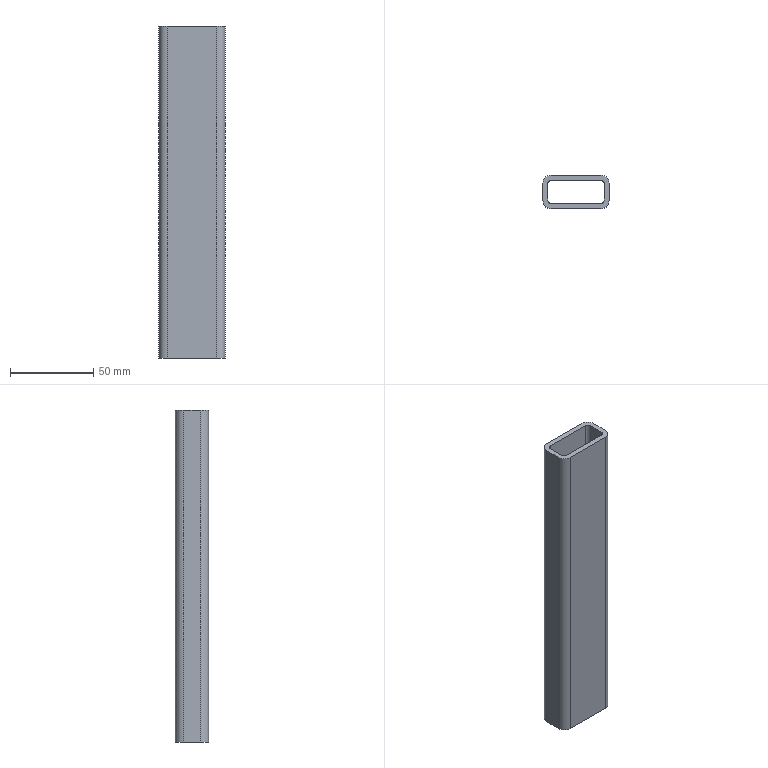Part | SolidWorks | features Extrusion 1 | 1 solid | 18 faces | box 40 x 20 x 200 mm | volume 61195 mm3 | plane 10 | cylinder 8 | commonest cylinder face diameters 4 x4 10 x4
STEP:
#1=CARTESIAN_POINT('',(35.,0.,200.));
#2=VERTEX_POINT('',#1);
#3=CARTESIAN_POINT('',(40.,5.,200.));
#4=VERTEX_POINT('',#3);
#5=CARTESIAN_POINT('',(35.,5.,200.));
#6=DIRECTION('',(0.,0.,1.));
#7=DIRECTION('',(1.,0.,0.));
#8=AXIS2_PLACEMENT_3D('',#5,#6,#7);
#9=CIRCLE('',#8,5.);
#10=EDGE_CURVE('',#2,#4,#9,.T.);
#11=ORIENTED_EDGE('',*,*,#10,.T.);
#12=CARTESIAN_POINT('',(40.,15.,200.));
#13=VERTEX_POINT('',#12);
#14=CARTESIAN_POINT('',(40.,5.,200.));
#15=DIRECTION('',(0.,1.,0.));
#16=VECTOR('',#15,1000.);
#17=LINE('',#14,#16);
#18=EDGE_CURVE('',#4,#13,#17,.T.);
#19=ORIENTED_EDGE('',*,*,#18,.T.);
#20=CARTESIAN_POINT('',(35.,20.,200.));
#21=VERTEX_POINT('',#20);
#22=CARTESIAN_POINT('',(35.,15.,200.));
#23=DIRECTION('',(0.,0.,1.));
#24=DIRECTION('',(-1.,0.,0.));
#25=AXIS2_PLACEMENT_3D('',#22,#23,#24);
#26=CIRCLE('',#25,5.);
#27=EDGE_CURVE('',#13,#21,#26,.T.);
#28=ORIENTED_EDGE('',*,*,#27,.T.);
#29=CARTESIAN_POINT('',(5.,20.,200.));
#30=VERTEX_POINT('',#29);
#31=CARTESIAN_POINT('',(5.,20.,200.));
#32=DIRECTION('',(-1.,0.,0.));
#33=VECTOR('',#32,1000.);
#34=LINE('',#31,#33);
#35=EDGE_CURVE('',#21,#30,#34,.T.);
#36=ORIENTED_EDGE('',*,*,#35,.T.);
#37=CARTESIAN_POINT('',(0.,15.,200.));
#38=VERTEX_POINT('',#37);
#39=CARTESIAN_POINT('',(5.,15.,200.));
#40=DIRECTION('',(0.,0.,1.));
#41=DIRECTION('',(-1.,0.,0.));
#42=AXIS2_PLACEMENT_3D('',#39,#40,#41);
#43=CIRCLE('',#42,5.);
#44=EDGE_CURVE('',#30,#38,#43,.T.);
#45=ORIENTED_EDGE('',*,*,#44,.T.);
#46=CARTESIAN_POINT('',(0.,5.,200.));
#47=VERTEX_POINT('',#46);
#48=CARTESIAN_POINT('',(0.,5.,200.));
#49=DIRECTION('',(0.,-1.,0.));
#50=VECTOR('',#49,1000.);
#51=LINE('',#48,#50);
#52=EDGE_CURVE('',#38,#47,#51,.T.);
#53=ORIENTED_EDGE('',*,*,#52,.T.);
#54=CARTESIAN_POINT('',(5.,0.,200.));
#55=VERTEX_POINT('',#54);
#56=CARTESIAN_POINT('',(5.,5.,200.));
#57=DIRECTION('',(0.,0.,1.));
#58=DIRECTION('',(-1.,0.,0.));
#59=AXIS2_PLACEMENT_3D('',#56,#57,#58);
#60=CIRCLE('',#59,5.);
#61=EDGE_CURVE('',#47,#55,#60,.T.);
#62=ORIENTED_EDGE('',*,*,#61,.T.);
#63=CARTESIAN_POINT('',(5.,0.,200.));
#64=DIRECTION('',(1.,0.,0.));
#65=VECTOR('',#64,1000.);
#66=LINE('',#63,#65);
#67=EDGE_CURVE('',#55,#2,#66,.T.);
#68=ORIENTED_EDGE('',*,*,#67,.T.);
#69=EDGE_LOOP('',(#11,#19,#28,#36,#45,#53,#62,#68));
#70=FACE_OUTER_BOUND('',#69,.T.);
#71=CARTESIAN_POINT('',(3.,15.,200.));
#72=VERTEX_POINT('',#71);
#73=CARTESIAN_POINT('',(3.,5.,200.));
#74=VERTEX_POINT('',#73);
#75=CARTESIAN_POINT('',(3.,5.,200.));
#76=DIRECTION('',(0.,-1.,0.));
#77=VECTOR('',#76,1000.);
#78=LINE('',#75,#77);
#79=EDGE_CURVE('',#72,#74,#78,.T.);
#80=ORIENTED_EDGE('',*,*,#79,.F.);
#81=CARTESIAN_POINT('',(5.,17.,200.));
#82=VERTEX_POINT('',#81);
#83=CARTESIAN_POINT('',(5.,15.,200.));
#84=DIRECTION('',(0.,0.,1.));
#85=DIRECTION('',(-1.,0.,0.));
#86=AXIS2_PLACEMENT_3D('',#83,#84,#85);
#87=CIRCLE('',#86,2.);
#88=EDGE_CURVE('',#82,#72,#87,.T.);
#89=ORIENTED_EDGE('',*,*,#88,.F.);
#90=CARTESIAN_POINT('',(35.,17.,200.));
#91=VERTEX_POINT('',#90);
#92=CARTESIAN_POINT('',(5.,17.,200.));
#93=DIRECTION('',(-1.,0.,0.));
#94=VECTOR('',#93,1000.);
#95=LINE('',#92,#94);
#96=EDGE_CURVE('',#91,#82,#95,.T.);
#97=ORIENTED_EDGE('',*,*,#96,.F.);
#98=CARTESIAN_POINT('',(37.,15.,200.));
#99=VERTEX_POINT('',#98);
#100=CARTESIAN_POINT('',(35.,15.,200.));
#101=DIRECTION('',(0.,0.,1.));
#102=DIRECTION('',(-1.,0.,0.));
#103=AXIS2_PLACEMENT_3D('',#100,#101,#102);
#104=CIRCLE('',#103,2.);
#105=EDGE_CURVE('',#99,#91,#104,.T.);
#106=ORIENTED_EDGE('',*,*,#105,.F.);
#107=CARTESIAN_POINT('',(37.,5.,200.));
#108=VERTEX_POINT('',#107);
#109=CARTESIAN_POINT('',(37.,5.,200.));
#110=DIRECTION('',(0.,1.,0.));
#111=VECTOR('',#110,1000.);
#112=LINE('',#109,#111);
#113=EDGE_CURVE('',#108,#99,#112,.T.);
#114=ORIENTED_EDGE('',*,*,#113,.F.);
#115=CARTESIAN_POINT('',(35.,3.,200.));
#116=VERTEX_POINT('',#115);
#117=CARTESIAN_POINT('',(35.,5.,200.));
#118=DIRECTION('',(0.,0.,1.));
#119=DIRECTION('',(1.,0.,0.));
#120=AXIS2_PLACEMENT_3D('',#117,#118,#119);
#121=CIRCLE('',#120,2.);
#122=EDGE_CURVE('',#116,#108,#121,.T.);
#123=ORIENTED_EDGE('',*,*,#122,.F.);
#124=CARTESIAN_POINT('',(5.,3.,200.));
#125=VERTEX_POINT('',#124);
#126=CARTESIAN_POINT('',(5.,3.,200.));
#127=DIRECTION('',(1.,0.,0.));
#128=VECTOR('',#127,1000.);
#129=LINE('',#126,#128);
#130=EDGE_CURVE('',#125,#116,#129,.T.);
#131=ORIENTED_EDGE('',*,*,#130,.F.);
#132=CARTESIAN_POINT('',(5.,5.,200.));
#133=DIRECTION('',(0.,0.,1.));
#134=DIRECTION('',(-1.,0.,0.));
#135=AXIS2_PLACEMENT_3D('',#132,#133,#134);
#136=CIRCLE('',#135,2.);
#137=EDGE_CURVE('',#74,#125,#136,.T.);
#138=ORIENTED_EDGE('',*,*,#137,.F.);
#139=EDGE_LOOP('',(#80,#89,#97,#106,#114,#123,#131,#138));
#140=FACE_BOUND('',#139,.T.);
#141=CARTESIAN_POINT('',(35.,5.,200.));
#142=DIRECTION('',(0.,0.,1.));
#143=DIRECTION('',(1.,0.,0.));
#144=AXIS2_PLACEMENT_3D('',#141,#142,#143);
#145=PLANE('',#144);
#146=ADVANCED_FACE('',(#70,#140),#145,.T.);
#147=CARTESIAN_POINT('',(35.,0.,0.));
#148=VERTEX_POINT('',#147);
#149=CARTESIAN_POINT('',(40.,5.,0.));
#150=VERTEX_POINT('',#149);
#151=CARTESIAN_POINT('',(35.,5.,0.));
#152=DIRECTION('',(0.,0.,1.));
#153=DIRECTION('',(1.,0.,0.));
#154=AXIS2_PLACEMENT_3D('',#151,#152,#153);
#155=CIRCLE('',#154,5.);
#156=EDGE_CURVE('',#148,#150,#155,.T.);
#157=ORIENTED_EDGE('',*,*,#156,.F.);
#158=CARTESIAN_POINT('',(5.,0.,0.));
#159=VERTEX_POINT('',#158);
#160=CARTESIAN_POINT('',(5.,0.,0.));
#161=DIRECTION('',(1.,0.,0.));
#162=VECTOR('',#161,1000.);
#163=LINE('',#160,#162);
#164=EDGE_CURVE('',#159,#148,#163,.T.);
#165=ORIENTED_EDGE('',*,*,#164,.F.);
#166=CARTESIAN_POINT('',(0.,5.,0.));
#167=VERTEX_POINT('',#166);
#168=CARTESIAN_POINT('',(5.,5.,0.));
#169=DIRECTION('',(0.,0.,1.));
#170=DIRECTION('',(-1.,0.,0.));
#171=AXIS2_PLACEMENT_3D('',#168,#169,#170);
#172=CIRCLE('',#171,5.);
#173=EDGE_CURVE('',#167,#159,#172,.T.);
#174=ORIENTED_EDGE('',*,*,#173,.F.);
#175=CARTESIAN_POINT('',(0.,15.,0.));
#176=VERTEX_POINT('',#175);
#177=CARTESIAN_POINT('',(0.,5.,0.));
#178=DIRECTION('',(0.,-1.,0.));
#179=VECTOR('',#178,1000.);
#180=LINE('',#177,#179);
#181=EDGE_CURVE('',#176,#167,#180,.T.);
#182=ORIENTED_EDGE('',*,*,#181,.F.);
#183=CARTESIAN_POINT('',(5.,20.,0.));
#184=VERTEX_POINT('',#183);
#185=CARTESIAN_POINT('',(5.,15.,0.));
#186=DIRECTION('',(0.,0.,1.));
#187=DIRECTION('',(-1.,0.,0.));
#188=AXIS2_PLACEMENT_3D('',#185,#186,#187);
#189=CIRCLE('',#188,5.);
#190=EDGE_CURVE('',#184,#176,#189,.T.);
#191=ORIENTED_EDGE('',*,*,#190,.F.);
#192=CARTESIAN_POINT('',(35.,20.,0.));
#193=VERTEX_POINT('',#192);
#194=CARTESIAN_POINT('',(5.,20.,0.));
#195=DIRECTION('',(-1.,0.,0.));
#196=VECTOR('',#195,1000.);
#197=LINE('',#194,#196);
#198=EDGE_CURVE('',#193,#184,#197,.T.);
#199=ORIENTED_EDGE('',*,*,#198,.F.);
#200=CARTESIAN_POINT('',(40.,15.,0.));
#201=VERTEX_POINT('',#200);
#202=CARTESIAN_POINT('',(35.,15.,0.));
#203=DIRECTION('',(0.,0.,1.));
#204=DIRECTION('',(-1.,0.,0.));
#205=AXIS2_PLACEMENT_3D('',#202,#203,#204);
#206=CIRCLE('',#205,5.);
#207=EDGE_CURVE('',#201,#193,#206,.T.);
#208=ORIENTED_EDGE('',*,*,#207,.F.);
#209=CARTESIAN_POINT('',(40.,5.,0.));
#210=DIRECTION('',(0.,1.,0.));
#211=VECTOR('',#210,1000.);
#212=LINE('',#209,#211);
#213=EDGE_CURVE('',#150,#201,#212,.T.);
#214=ORIENTED_EDGE('',*,*,#213,.F.);
#215=EDGE_LOOP('',(#157,#165,#174,#182,#191,#199,#208,#214));
#216=FACE_OUTER_BOUND('',#215,.T.);
#217=CARTESIAN_POINT('',(5.,17.,0.));
#218=VERTEX_POINT('',#217);
#219=CARTESIAN_POINT('',(3.,15.,0.));
#220=VERTEX_POINT('',#219);
#221=CARTESIAN_POINT('',(5.,15.,0.));
#222=DIRECTION('',(0.,0.,1.));
#223=DIRECTION('',(-1.,0.,0.));
#224=AXIS2_PLACEMENT_3D('',#221,#222,#223);
#225=CIRCLE('',#224,2.);
#226=EDGE_CURVE('',#218,#220,#225,.T.);
#227=ORIENTED_EDGE('',*,*,#226,.T.);
#228=CARTESIAN_POINT('',(3.,5.,0.));
#229=VERTEX_POINT('',#228);
#230=CARTESIAN_POINT('',(3.,5.,0.));
#231=DIRECTION('',(0.,-1.,0.));
#232=VECTOR('',#231,1000.);
#233=LINE('',#230,#232);
#234=EDGE_CURVE('',#220,#229,#233,.T.);
#235=ORIENTED_EDGE('',*,*,#234,.T.);
#236=CARTESIAN_POINT('',(5.,3.,0.));
#237=VERTEX_POINT('',#236);
#238=CARTESIAN_POINT('',(5.,5.,0.));
#239=DIRECTION('',(0.,0.,1.));
#240=DIRECTION('',(-1.,0.,0.));
#241=AXIS2_PLACEMENT_3D('',#238,#239,#240);
#242=CIRCLE('',#241,2.);
#243=EDGE_CURVE('',#229,#237,#242,.T.);
#244=ORIENTED_EDGE('',*,*,#243,.T.);
#245=CARTESIAN_POINT('',(35.,3.,0.));
#246=VERTEX_POINT('',#245);
#247=CARTESIAN_POINT('',(5.,3.,0.));
#248=DIRECTION('',(1.,0.,0.));
#249=VECTOR('',#248,1000.);
#250=LINE('',#247,#249);
#251=EDGE_CURVE('',#237,#246,#250,.T.);
#252=ORIENTED_EDGE('',*,*,#251,.T.);
#253=CARTESIAN_POINT('',(37.,5.,0.));
#254=VERTEX_POINT('',#253);
#255=CARTESIAN_POINT('',(35.,5.,0.));
#256=DIRECTION('',(0.,0.,1.));
#257=DIRECTION('',(1.,0.,0.));
#258=AXIS2_PLACEMENT_3D('',#255,#256,#257);
#259=CIRCLE('',#258,2.);
#260=EDGE_CURVE('',#246,#254,#259,.T.);
#261=ORIENTED_EDGE('',*,*,#260,.T.);
#262=CARTESIAN_POINT('',(37.,15.,0.));
#263=VERTEX_POINT('',#262);
#264=CARTESIAN_POINT('',(37.,5.,0.));
#265=DIRECTION('',(0.,1.,0.));
#266=VECTOR('',#265,1000.);
#267=LINE('',#264,#266);
#268=EDGE_CURVE('',#254,#263,#267,.T.);
#269=ORIENTED_EDGE('',*,*,#268,.T.);
#270=CARTESIAN_POINT('',(35.,17.,0.));
#271=VERTEX_POINT('',#270);
#272=CARTESIAN_POINT('',(35.,15.,0.));
#273=DIRECTION('',(0.,0.,1.));
#274=DIRECTION('',(-1.,0.,0.));
#275=AXIS2_PLACEMENT_3D('',#272,#273,#274);
#276=CIRCLE('',#275,2.);
#277=EDGE_CURVE('',#263,#271,#276,.T.);
#278=ORIENTED_EDGE('',*,*,#277,.T.);
#279=CARTESIAN_POINT('',(5.,17.,0.));
#280=DIRECTION('',(-1.,0.,0.));
#281=VECTOR('',#280,1000.);
#282=LINE('',#279,#281);
#283=EDGE_CURVE('',#271,#218,#282,.T.);
#284=ORIENTED_EDGE('',*,*,#283,.T.);
#285=EDGE_LOOP('',(#227,#235,#244,#252,#261,#269,#278,#284));
#286=FACE_BOUND('',#285,.T.);
#287=CARTESIAN_POINT('',(35.,5.,0.));
#288=DIRECTION('',(0.,0.,1.));
#289=DIRECTION('',(1.,0.,0.));
#290=AXIS2_PLACEMENT_3D('',#287,#288,#289);
#291=PLANE('',#290);
#292=ADVANCED_FACE('',(#216,#286),#291,.F.);
#293=ORIENTED_EDGE('',*,*,#156,.T.);
#294=CARTESIAN_POINT('',(40.,5.,200.));
#295=DIRECTION('',(0.,0.,-1.));
#296=VECTOR('',#295,1000.);
#297=LINE('',#294,#296);
#298=EDGE_CURVE('',#4,#150,#297,.T.);
#299=ORIENTED_EDGE('',*,*,#298,.F.);
#300=ORIENTED_EDGE('',*,*,#10,.F.);
#301=CARTESIAN_POINT('',(35.,0.,200.));
#302=DIRECTION('',(0.,0.,-1.));
#303=VECTOR('',#302,1000.);
#304=LINE('',#301,#303);
#305=EDGE_CURVE('',#2,#148,#304,.T.);
#306=ORIENTED_EDGE('',*,*,#305,.T.);
#307=EDGE_LOOP('',(#293,#299,#300,#306));
#308=FACE_OUTER_BOUND('',#307,.T.);
#309=CARTESIAN_POINT('',(35.,5.,200.));
#310=DIRECTION('',(0.,0.,-1.));
#311=DIRECTION('',(-1.,0.,0.));
#312=AXIS2_PLACEMENT_3D('',#309,#310,#311);
#313=CYLINDRICAL_SURFACE('',#312,5.);
#314=ADVANCED_FACE('',(#308),#313,.T.);
#315=ORIENTED_EDGE('',*,*,#213,.T.);
#316=CARTESIAN_POINT('',(40.,15.,200.));
#317=DIRECTION('',(0.,0.,-1.));
#318=VECTOR('',#317,1000.);
#319=LINE('',#316,#318);
#320=EDGE_CURVE('',#13,#201,#319,.T.);
#321=ORIENTED_EDGE('',*,*,#320,.F.);
#322=ORIENTED_EDGE('',*,*,#18,.F.);
#323=ORIENTED_EDGE('',*,*,#298,.T.);
#324=EDGE_LOOP('',(#315,#321,#322,#323));
#325=FACE_OUTER_BOUND('',#324,.T.);
#326=CARTESIAN_POINT('',(40.,5.,200.));
#327=DIRECTION('',(-1.,0.,0.));
#328=DIRECTION('',(0.,0.,1.));
#329=AXIS2_PLACEMENT_3D('',#326,#327,#328);
#330=PLANE('',#329);
#331=ADVANCED_FACE('',(#325),#330,.F.);
#332=ORIENTED_EDGE('',*,*,#207,.T.);
#333=CARTESIAN_POINT('',(35.,20.,200.));
#334=DIRECTION('',(0.,0.,-1.));
#335=VECTOR('',#334,1000.);
#336=LINE('',#333,#335);
#337=EDGE_CURVE('',#21,#193,#336,.T.);
#338=ORIENTED_EDGE('',*,*,#337,.F.);
#339=ORIENTED_EDGE('',*,*,#27,.F.);
#340=ORIENTED_EDGE('',*,*,#320,.T.);
#341=EDGE_LOOP('',(#332,#338,#339,#340));
#342=FACE_OUTER_BOUND('',#341,.T.);
#343=CARTESIAN_POINT('',(35.,15.,200.));
#344=DIRECTION('',(0.,0.,-1.));
#345=DIRECTION('',(-1.,0.,0.));
#346=AXIS2_PLACEMENT_3D('',#343,#344,#345);
#347=CYLINDRICAL_SURFACE('',#346,5.);
#348=ADVANCED_FACE('',(#342),#347,.T.);
#349=ORIENTED_EDGE('',*,*,#198,.T.);
#350=CARTESIAN_POINT('',(5.,20.,200.));
#351=DIRECTION('',(0.,0.,-1.));
#352=VECTOR('',#351,1000.);
#353=LINE('',#350,#352);
#354=EDGE_CURVE('',#30,#184,#353,.T.);
#355=ORIENTED_EDGE('',*,*,#354,.F.);
#356=ORIENTED_EDGE('',*,*,#35,.F.);
#357=ORIENTED_EDGE('',*,*,#337,.T.);
#358=EDGE_LOOP('',(#349,#355,#356,#357));
#359=FACE_OUTER_BOUND('',#358,.T.);
#360=CARTESIAN_POINT('',(5.,20.,200.));
#361=DIRECTION('',(0.,-1.,0.));
#362=DIRECTION('',(0.,0.,-1.));
#363=AXIS2_PLACEMENT_3D('',#360,#361,#362);
#364=PLANE('',#363);
#365=ADVANCED_FACE('',(#359),#364,.F.);
#366=ORIENTED_EDGE('',*,*,#190,.T.);
#367=CARTESIAN_POINT('',(0.,15.,200.));
#368=DIRECTION('',(0.,0.,-1.));
#369=VECTOR('',#368,1000.);
#370=LINE('',#367,#369);
#371=EDGE_CURVE('',#38,#176,#370,.T.);
#372=ORIENTED_EDGE('',*,*,#371,.F.);
#373=ORIENTED_EDGE('',*,*,#44,.F.);
#374=ORIENTED_EDGE('',*,*,#354,.T.);
#375=EDGE_LOOP('',(#366,#372,#373,#374));
#376=FACE_OUTER_BOUND('',#375,.T.);
#377=CARTESIAN_POINT('',(5.,15.,200.));
#378=DIRECTION('',(0.,0.,-1.));
#379=DIRECTION('',(-1.,0.,0.));
#380=AXIS2_PLACEMENT_3D('',#377,#378,#379);
#381=CYLINDRICAL_SURFACE('',#380,5.);
#382=ADVANCED_FACE('',(#376),#381,.T.);
#383=ORIENTED_EDGE('',*,*,#181,.T.);
#384=CARTESIAN_POINT('',(0.,5.,200.));
#385=DIRECTION('',(0.,0.,-1.));
#386=VECTOR('',#385,1000.);
#387=LINE('',#384,#386);
#388=EDGE_CURVE('',#47,#167,#387,.T.);
#389=ORIENTED_EDGE('',*,*,#388,.F.);
#390=ORIENTED_EDGE('',*,*,#52,.F.);
#391=ORIENTED_EDGE('',*,*,#371,.T.);
#392=EDGE_LOOP('',(#383,#389,#390,#391));
#393=FACE_OUTER_BOUND('',#392,.T.);
#394=CARTESIAN_POINT('',(0.,5.,200.));
#395=DIRECTION('',(1.,0.,0.));
#396=DIRECTION('',(0.,0.,-1.));
#397=AXIS2_PLACEMENT_3D('',#394,#395,#396);
#398=PLANE('',#397);
#399=ADVANCED_FACE('',(#393),#398,.F.);
#400=ORIENTED_EDGE('',*,*,#173,.T.);
#401=CARTESIAN_POINT('',(5.,0.,200.));
#402=DIRECTION('',(0.,0.,-1.));
#403=VECTOR('',#402,1000.);
#404=LINE('',#401,#403);
#405=EDGE_CURVE('',#55,#159,#404,.T.);
#406=ORIENTED_EDGE('',*,*,#405,.F.);
#407=ORIENTED_EDGE('',*,*,#61,.F.);
#408=ORIENTED_EDGE('',*,*,#388,.T.);
#409=EDGE_LOOP('',(#400,#406,#407,#408));
#410=FACE_OUTER_BOUND('',#409,.T.);
#411=CARTESIAN_POINT('',(5.,5.,200.));
#412=DIRECTION('',(0.,0.,-1.));
#413=DIRECTION('',(-1.,0.,0.));
#414=AXIS2_PLACEMENT_3D('',#411,#412,#413);
#415=CYLINDRICAL_SURFACE('',#414,5.);
#416=ADVANCED_FACE('',(#410),#415,.T.);
#417=ORIENTED_EDGE('',*,*,#164,.T.);
#418=ORIENTED_EDGE('',*,*,#305,.F.);
#419=ORIENTED_EDGE('',*,*,#67,.F.);
#420=ORIENTED_EDGE('',*,*,#405,.T.);
#421=EDGE_LOOP('',(#417,#418,#419,#420));
#422=FACE_OUTER_BOUND('',#421,.T.);
#423=CARTESIAN_POINT('',(5.,0.,200.));
#424=DIRECTION('',(0.,1.,0.));
#425=DIRECTION('',(0.,0.,1.));
#426=AXIS2_PLACEMENT_3D('',#423,#424,#425);
#427=PLANE('',#426);
#428=ADVANCED_FACE('',(#422),#427,.F.);
#429=ORIENTED_EDGE('',*,*,#226,.F.);
#430=CARTESIAN_POINT('',(5.,17.,200.));
#431=DIRECTION('',(0.,0.,-1.));
#432=VECTOR('',#431,1000.);
#433=LINE('',#430,#432);
#434=EDGE_CURVE('',#82,#218,#433,.T.);
#435=ORIENTED_EDGE('',*,*,#434,.F.);
#436=ORIENTED_EDGE('',*,*,#88,.T.);
#437=CARTESIAN_POINT('',(3.,15.,200.));
#438=DIRECTION('',(0.,0.,-1.));
#439=VECTOR('',#438,1000.);
#440=LINE('',#437,#439);
#441=EDGE_CURVE('',#72,#220,#440,.T.);
#442=ORIENTED_EDGE('',*,*,#441,.T.);
#443=EDGE_LOOP('',(#429,#435,#436,#442));
#444=FACE_OUTER_BOUND('',#443,.T.);
#445=CARTESIAN_POINT('',(5.,15.,200.));
#446=DIRECTION('',(0.,0.,-1.));
#447=DIRECTION('',(-1.,0.,0.));
#448=AXIS2_PLACEMENT_3D('',#445,#446,#447);
#449=CYLINDRICAL_SURFACE('',#448,2.);
#450=ADVANCED_FACE('',(#444),#449,.F.);
#451=ORIENTED_EDGE('',*,*,#234,.F.);
#452=ORIENTED_EDGE('',*,*,#441,.F.);
#453=ORIENTED_EDGE('',*,*,#79,.T.);
#454=CARTESIAN_POINT('',(3.,5.,200.));
#455=DIRECTION('',(0.,0.,-1.));
#456=VECTOR('',#455,1000.);
#457=LINE('',#454,#456);
#458=EDGE_CURVE('',#74,#229,#457,.T.);
#459=ORIENTED_EDGE('',*,*,#458,.T.);
#460=EDGE_LOOP('',(#451,#452,#453,#459));
#461=FACE_OUTER_BOUND('',#460,.T.);
#462=CARTESIAN_POINT('',(3.,5.,200.));
#463=DIRECTION('',(1.,0.,0.));
#464=DIRECTION('',(0.,0.,-1.));
#465=AXIS2_PLACEMENT_3D('',#462,#463,#464);
#466=PLANE('',#465);
#467=ADVANCED_FACE('',(#461),#466,.T.);
#468=ORIENTED_EDGE('',*,*,#243,.F.);
#469=ORIENTED_EDGE('',*,*,#458,.F.);
#470=ORIENTED_EDGE('',*,*,#137,.T.);
#471=CARTESIAN_POINT('',(5.,3.,200.));
#472=DIRECTION('',(0.,0.,-1.));
#473=VECTOR('',#472,1000.);
#474=LINE('',#471,#473);
#475=EDGE_CURVE('',#125,#237,#474,.T.);
#476=ORIENTED_EDGE('',*,*,#475,.T.);
#477=EDGE_LOOP('',(#468,#469,#470,#476));
#478=FACE_OUTER_BOUND('',#477,.T.);
#479=CARTESIAN_POINT('',(5.,5.,200.));
#480=DIRECTION('',(0.,0.,-1.));
#481=DIRECTION('',(-1.,0.,0.));
#482=AXIS2_PLACEMENT_3D('',#479,#480,#481);
#483=CYLINDRICAL_SURFACE('',#482,2.);
#484=ADVANCED_FACE('',(#478),#483,.F.);
#485=ORIENTED_EDGE('',*,*,#251,.F.);
#486=ORIENTED_EDGE('',*,*,#475,.F.);
#487=ORIENTED_EDGE('',*,*,#130,.T.);
#488=CARTESIAN_POINT('',(35.,3.,200.));
#489=DIRECTION('',(0.,0.,-1.));
#490=VECTOR('',#489,1000.);
#491=LINE('',#488,#490);
#492=EDGE_CURVE('',#116,#246,#491,.T.);
#493=ORIENTED_EDGE('',*,*,#492,.T.);
#494=EDGE_LOOP('',(#485,#486,#487,#493));
#495=FACE_OUTER_BOUND('',#494,.T.);
#496=CARTESIAN_POINT('',(5.,3.,200.));
#497=DIRECTION('',(0.,1.,0.));
#498=DIRECTION('',(-1.,0.,0.));
#499=AXIS2_PLACEMENT_3D('',#496,#497,#498);
#500=PLANE('',#499);
#501=ADVANCED_FACE('',(#495),#500,.T.);
#502=ORIENTED_EDGE('',*,*,#260,.F.);
#503=ORIENTED_EDGE('',*,*,#492,.F.);
#504=ORIENTED_EDGE('',*,*,#122,.T.);
#505=CARTESIAN_POINT('',(37.,5.,200.));
#506=DIRECTION('',(0.,0.,-1.));
#507=VECTOR('',#506,1000.);
#508=LINE('',#505,#507);
#509=EDGE_CURVE('',#108,#254,#508,.T.);
#510=ORIENTED_EDGE('',*,*,#509,.T.);
#511=EDGE_LOOP('',(#502,#503,#504,#510));
#512=FACE_OUTER_BOUND('',#511,.T.);
#513=CARTESIAN_POINT('',(35.,5.,200.));
#514=DIRECTION('',(0.,0.,-1.));
#515=DIRECTION('',(-1.,0.,0.));
#516=AXIS2_PLACEMENT_3D('',#513,#514,#515);
#517=CYLINDRICAL_SURFACE('',#516,2.);
#518=ADVANCED_FACE('',(#512),#517,.F.);
#519=ORIENTED_EDGE('',*,*,#268,.F.);
#520=ORIENTED_EDGE('',*,*,#509,.F.);
#521=ORIENTED_EDGE('',*,*,#113,.T.);
#522=CARTESIAN_POINT('',(37.,15.,200.));
#523=DIRECTION('',(0.,0.,-1.));
#524=VECTOR('',#523,1000.);
#525=LINE('',#522,#524);
#526=EDGE_CURVE('',#99,#263,#525,.T.);
#527=ORIENTED_EDGE('',*,*,#526,.T.);
#528=EDGE_LOOP('',(#519,#520,#521,#527));
#529=FACE_OUTER_BOUND('',#528,.T.);
#530=CARTESIAN_POINT('',(37.,5.,200.));
#531=DIRECTION('',(-1.,0.,0.));
#532=DIRECTION('',(0.,-1.,0.));
#533=AXIS2_PLACEMENT_3D('',#530,#531,#532);
#534=PLANE('',#533);
#535=ADVANCED_FACE('',(#529),#534,.T.);
#536=ORIENTED_EDGE('',*,*,#277,.F.);
#537=ORIENTED_EDGE('',*,*,#526,.F.);
#538=ORIENTED_EDGE('',*,*,#105,.T.);
#539=CARTESIAN_POINT('',(35.,17.,200.));
#540=DIRECTION('',(0.,0.,-1.));
#541=VECTOR('',#540,1000.);
#542=LINE('',#539,#541);
#543=EDGE_CURVE('',#91,#271,#542,.T.);
#544=ORIENTED_EDGE('',*,*,#543,.T.);
#545=EDGE_LOOP('',(#536,#537,#538,#544));
#546=FACE_OUTER_BOUND('',#545,.T.);
#547=CARTESIAN_POINT('',(35.,15.,200.));
#548=DIRECTION('',(0.,0.,-1.));
#549=DIRECTION('',(-1.,0.,0.));
#550=AXIS2_PLACEMENT_3D('',#547,#548,#549);
#551=CYLINDRICAL_SURFACE('',#550,2.);
#552=ADVANCED_FACE('',(#546),#551,.F.);
#553=ORIENTED_EDGE('',*,*,#283,.F.);
#554=ORIENTED_EDGE('',*,*,#543,.F.);
#555=ORIENTED_EDGE('',*,*,#96,.T.);
#556=ORIENTED_EDGE('',*,*,#434,.T.);
#557=EDGE_LOOP('',(#553,#554,#555,#556));
#558=FACE_OUTER_BOUND('',#557,.T.);
#559=CARTESIAN_POINT('',(5.,17.,200.));
#560=DIRECTION('',(0.,-1.,0.));
#561=DIRECTION('',(0.,0.,-1.));
#562=AXIS2_PLACEMENT_3D('',#559,#560,#561);
#563=PLANE('',#562);
#564=ADVANCED_FACE('',(#558),#563,.T.);
#565=CLOSED_SHELL('',(#146,#292,#314,#331,#348,#365,#382,#399,#416,#428,#450,#467,#484,#501,#518,#535,#552,#564));
#566=MANIFOLD_SOLID_BREP('',#565);
#567=CARTESIAN_POINT('',(0.,0.,0.));
#568=DIRECTION('',(0.,0.,1.));
#569=DIRECTION('',(1.,0.,0.));
#570=AXIS2_PLACEMENT_3D('',#567,#568,#569);
#571=(LENGTH_UNIT()NAMED_UNIT(*)SI_UNIT(.MILLI.,.METRE.));
#572=UNCERTAINTY_MEASURE_WITH_UNIT(LENGTH_MEASURE(0.00001),#571,'','');
#573=(NAMED_UNIT(*)PLANE_ANGLE_UNIT()SI_UNIT($,.RADIAN.));
#574=(NAMED_UNIT(*)SI_UNIT($,.STERADIAN.)SOLID_ANGLE_UNIT());
#575=(GEOMETRIC_REPRESENTATION_CONTEXT(3)GLOBAL_UNCERTAINTY_ASSIGNED_CONTEXT((#572))GLOBAL_UNIT_ASSIGNED_CONTEXT((#571,#573,#574))REPRESENTATION_CONTEXT('',''));
#576=ADVANCED_BREP_SHAPE_REPRESENTATION('',(#566,#570),#575);